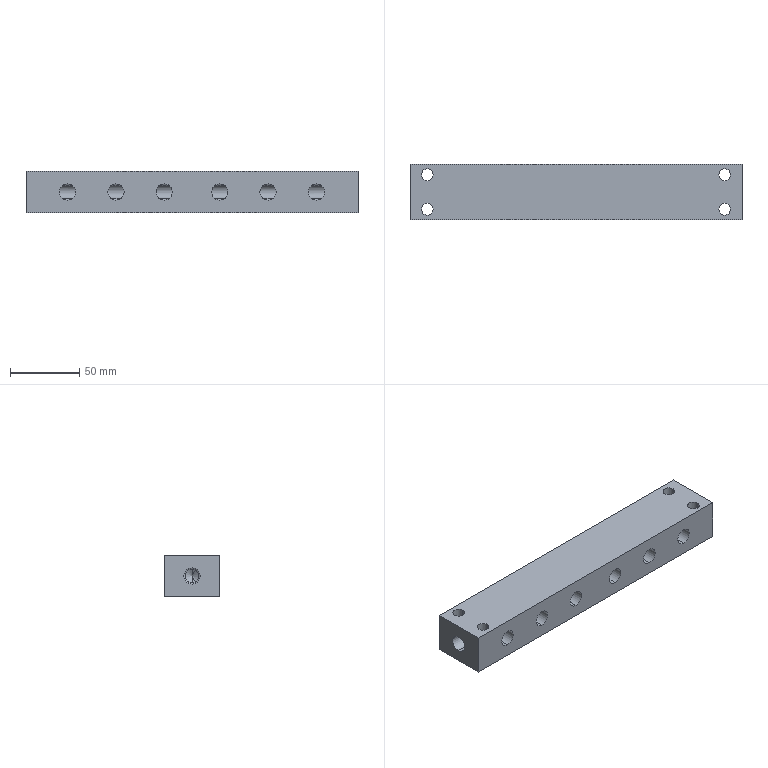Part | SolidWorks | features HoleWzd 6, MirrorPattern 2, Extrusion 1 | 1 solid | 78 faces | box 240 x 40 x 30 mm | volume 239495 mm3 | cylinder 42 | cone 30 | plane 6 | commonest cylinder face diameters 11.8 x16 10 x14 8.5 x8 19 x4